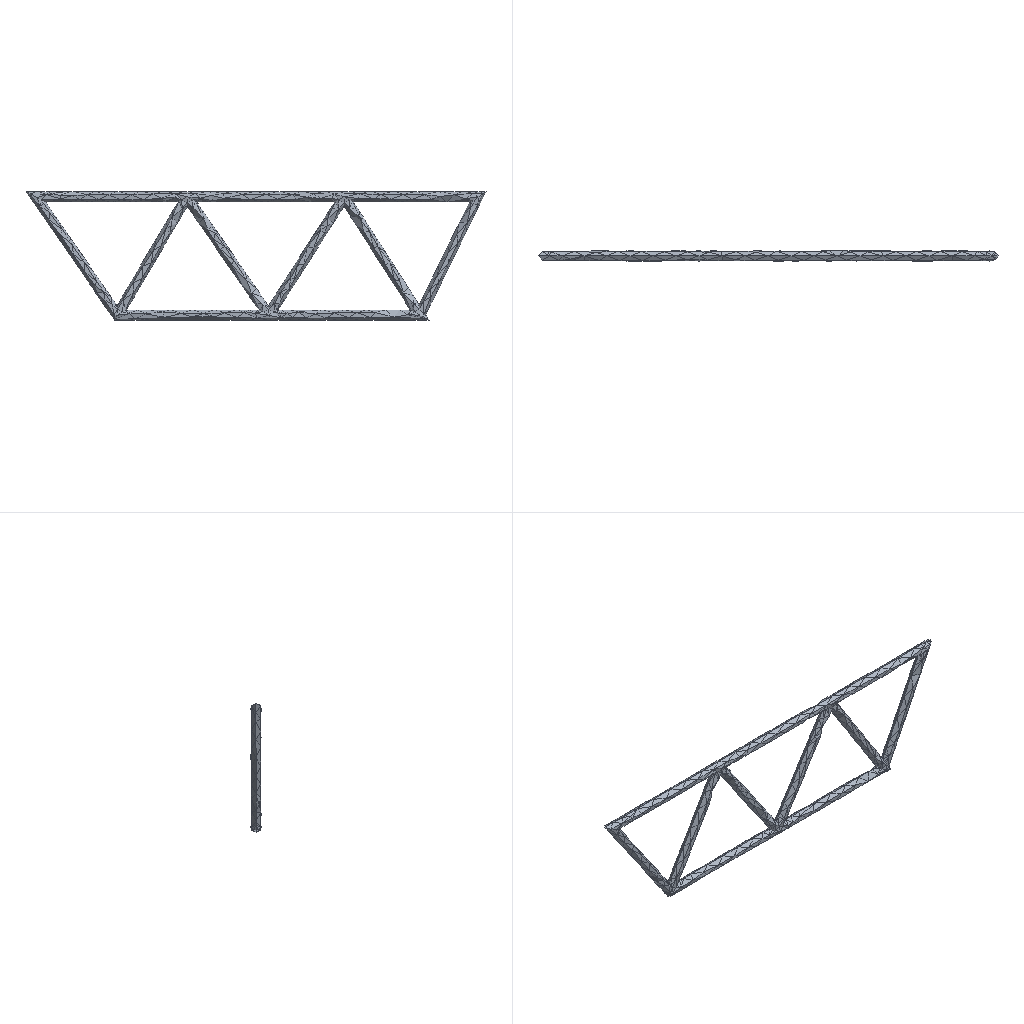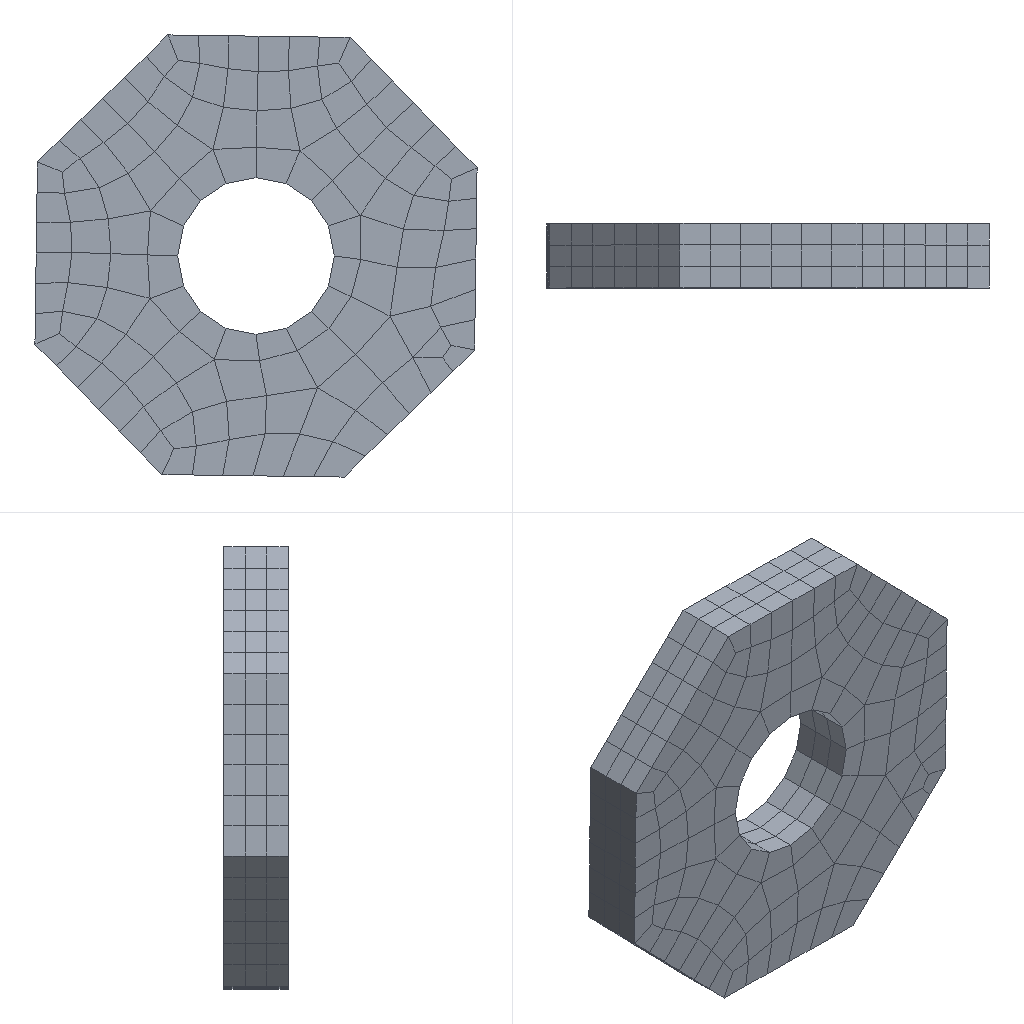Simulation study | ansys workbench
Set-up summary:
category,name,step,type,value,unit,region
solver,ansys_mapdl
solver,version,,,22.1
solver,version,,,22.1
solver,version,,,22.1
units,MPA,,stated
analysis,deck1,,static,static
load_step,requested,,,1
analysis,nlgeom,,,False
mesh,nodes,,,99
mesh,elements,,,68
element_type,ANSYS 188 (type 1),,beam,14
element_type,ANSYS 188 (type 2),,beam,20
element_type,ANSYS 188 (type 3),,beam,14
element_type,ANSYS 156 (type 4),,surface,20
load,load commands in deck,,count,3
bc,support commands in deck,,count,1
named_set,_ELMISC,,component
named_set,_FIXEDSU,,component
analysis,deck2,,static,static
load_step,requested,,,1
analysis,nlgeom,,,False
mesh,nodes,,,2182
mesh,elements,,,414
element_type,ANSYS 186 (type 1),,solid,366
element_type,ANSYS 154 (type 2),,surface,48
load,load commands in deck,,count,3
bc,support commands in deck,,count,1
named_set,_FIXEDSU,,component
analysis,deck3,,static,static
load_step,requested,,,1
analysis,nlgeom,,,False
mesh,nodes,,,3646
mesh,elements,,,2089
element_type,ANSYS 187 (type 1),,solid,1681
element_type,ANSYS 154 (type 2),,surface,408
load,load commands in deck,,count,3
bc,support commands in deck,,count,1
named_set,_FIXEDSU,,component
material,1,,in results
material,2,,in results
material,3,,in results
material,1,,in results
material,1,,in results
check,setup vs results,,match,"48 beam element(s) were compared without their orientation node (the deck's third node, which no element of the results uses); 48 node(s) the solver created internally for pilot nodes (ansys-fenxi-4/桥梁分析/桥梁_files/dp0/SYS-1/MECH/solve.out) are in the results only; 20 surface effect element(s) are not in the reader's mesh and were not compared"
check,setup vs results,,match,48 surface effect element(s) are not in the reader's mesh and were not compared
check,setup vs results,,match,408 surface effect element(s) are not in the reader's mesh and were not compared
Results summary:
result,analysis,,,static
result,last_loadstep,,,1
result,primary field,,,displacement
result,reaction total,1,FX,-0.0,N
result,reaction total,1,FY,0.0,N
result,reaction total,1,FZ,-93.0,N
result,mass,,,0.0,"NMM: mm, ton, N, s, mV, mA, degC"
result,analysis,,,static
result,last_loadstep,,,1
result,primary field,,,displacement
result,reaction total,1,FX,-93.0,N
result,reaction total,1,FY,-93.0,N
result,reaction total,1,FZ,-93.0,N
result,mass,,,0.000267,"NMM: mm, ton, N, s, mV, mA, degC"
result,analysis,,,static
result,last_loadstep,,,1
result,primary field,,,displacement
result,reaction total,1,FX,0.0,N
result,reaction total,1,FY,-0.0,N
result,reaction total,1,FZ,-92.949,N
result,mass,,,14.221,"NMM: mm, ton, N, s, mV, mA, degC"